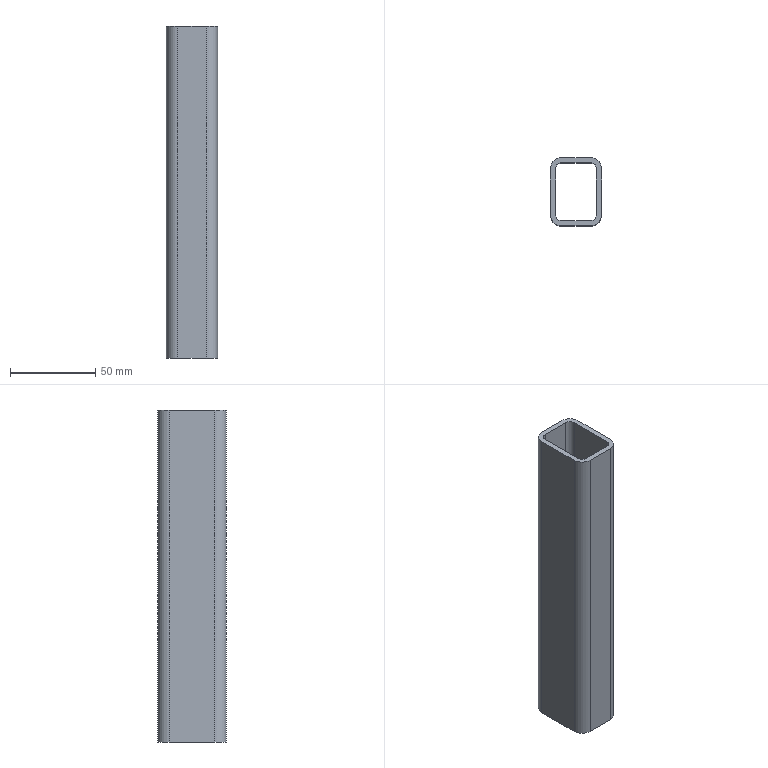Part | STEP file | DIN EN 10305-5 40 x 30 x 3 1785429668101 | 1 solid | 18 faces | box 30 x 40 x 194.434 mm | volume 69555 mm3 | plane 10 | cylinder 8 | commonest cylinder face diameters 7.2 x4 13.2 x4
STEP:
#1=CARTESIAN_POINT('',(-8.4,-17.,194.434));
#2=VERTEX_POINT('',#1);
#3=CARTESIAN_POINT('',(8.4,-17.,194.434));
#4=VERTEX_POINT('',#3);
#5=CARTESIAN_POINT('',(4.2,-17.,194.434));
#6=DIRECTION('',(1.,0.,0.));
#7=VECTOR('',#6,10.);
#8=LINE('',#5,#7);
#9=EDGE_CURVE('',#2,#4,#8,.T.);
#10=ORIENTED_EDGE('',*,*,#9,.T.);
#11=CARTESIAN_POINT('',(8.4,-17.,0.));
#12=VERTEX_POINT('',#11);
#13=CARTESIAN_POINT('',(8.4,-17.,0.));
#14=DIRECTION('',(0.,0.,1.));
#15=VECTOR('',#14,10.);
#16=LINE('',#13,#15);
#17=EDGE_CURVE('',#12,#4,#16,.T.);
#18=ORIENTED_EDGE('',*,*,#17,.F.);
#19=CARTESIAN_POINT('',(-8.4,-17.,0.));
#20=VERTEX_POINT('',#19);
#21=CARTESIAN_POINT('',(4.2,-17.,0.));
#22=DIRECTION('',(1.,0.,0.));
#23=VECTOR('',#22,10.);
#24=LINE('',#21,#23);
#25=EDGE_CURVE('',#20,#12,#24,.T.);
#26=ORIENTED_EDGE('',*,*,#25,.F.);
#27=CARTESIAN_POINT('',(-8.4,-17.,0.));
#28=DIRECTION('',(0.,0.,1.));
#29=VECTOR('',#28,10.);
#30=LINE('',#27,#29);
#31=EDGE_CURVE('',#20,#2,#30,.T.);
#32=ORIENTED_EDGE('',*,*,#31,.T.);
#33=EDGE_LOOP('',(#10,#18,#26,#32));
#34=FACE_OUTER_BOUND('',#33,.T.);
#35=CARTESIAN_POINT('',(8.4,-17.,0.));
#36=DIRECTION('',(0.,-1.,0.));
#37=DIRECTION('',(0.,0.,-1.));
#38=AXIS2_PLACEMENT_3D('',#35,#36,#37);
#39=PLANE('',#38);
#40=ADVANCED_FACE('',(#34),#39,.F.);
#41=CARTESIAN_POINT('',(12.,-13.4,194.434));
#42=VERTEX_POINT('',#41);
#43=CARTESIAN_POINT('',(8.4,-13.4,194.434));
#44=DIRECTION('',(0.,0.,1.));
#45=DIRECTION('',(0.,1.,0.));
#46=AXIS2_PLACEMENT_3D('',#43,#44,#45);
#47=CIRCLE('',#46,3.6);
#48=EDGE_CURVE('',#4,#42,#47,.T.);
#49=ORIENTED_EDGE('',*,*,#48,.T.);
#50=CARTESIAN_POINT('',(12.,-13.4,0.));
#51=VERTEX_POINT('',#50);
#52=CARTESIAN_POINT('',(12.,-13.4,0.));
#53=DIRECTION('',(0.,0.,1.));
#54=VECTOR('',#53,10.);
#55=LINE('',#52,#54);
#56=EDGE_CURVE('',#51,#42,#55,.T.);
#57=ORIENTED_EDGE('',*,*,#56,.F.);
#58=CARTESIAN_POINT('',(8.4,-13.4,0.));
#59=DIRECTION('',(0.,0.,1.));
#60=DIRECTION('',(0.,1.,0.));
#61=AXIS2_PLACEMENT_3D('',#58,#59,#60);
#62=CIRCLE('',#61,3.6);
#63=EDGE_CURVE('',#12,#51,#62,.T.);
#64=ORIENTED_EDGE('',*,*,#63,.F.);
#65=ORIENTED_EDGE('',*,*,#17,.T.);
#66=EDGE_LOOP('',(#49,#57,#64,#65));
#67=FACE_OUTER_BOUND('',#66,.T.);
#68=CARTESIAN_POINT('',(8.4,-13.4,0.));
#69=DIRECTION('',(0.,0.,1.));
#70=DIRECTION('',(0.,1.,0.));
#71=AXIS2_PLACEMENT_3D('',#68,#69,#70);
#72=CYLINDRICAL_SURFACE('',#71,3.6);
#73=ADVANCED_FACE('',(#67),#72,.F.);
#74=CARTESIAN_POINT('',(12.,13.4,194.434));
#75=VERTEX_POINT('',#74);
#76=CARTESIAN_POINT('',(12.,6.7,194.434));
#77=DIRECTION('',(0.,1.,0.));
#78=VECTOR('',#77,10.);
#79=LINE('',#76,#78);
#80=EDGE_CURVE('',#42,#75,#79,.T.);
#81=ORIENTED_EDGE('',*,*,#80,.T.);
#82=CARTESIAN_POINT('',(12.,13.4,0.));
#83=VERTEX_POINT('',#82);
#84=CARTESIAN_POINT('',(12.,13.4,0.));
#85=DIRECTION('',(0.,0.,1.));
#86=VECTOR('',#85,10.);
#87=LINE('',#84,#86);
#88=EDGE_CURVE('',#83,#75,#87,.T.);
#89=ORIENTED_EDGE('',*,*,#88,.F.);
#90=CARTESIAN_POINT('',(12.,6.7,0.));
#91=DIRECTION('',(0.,1.,0.));
#92=VECTOR('',#91,10.);
#93=LINE('',#90,#92);
#94=EDGE_CURVE('',#51,#83,#93,.T.);
#95=ORIENTED_EDGE('',*,*,#94,.F.);
#96=ORIENTED_EDGE('',*,*,#56,.T.);
#97=EDGE_LOOP('',(#81,#89,#95,#96));
#98=FACE_OUTER_BOUND('',#97,.T.);
#99=CARTESIAN_POINT('',(12.,13.4,0.));
#100=DIRECTION('',(1.,0.,0.));
#101=DIRECTION('',(0.,0.,-1.));
#102=AXIS2_PLACEMENT_3D('',#99,#100,#101);
#103=PLANE('',#102);
#104=ADVANCED_FACE('',(#98),#103,.F.);
#105=CARTESIAN_POINT('',(8.4,17.,194.434));
#106=VERTEX_POINT('',#105);
#107=CARTESIAN_POINT('',(8.4,13.4,194.434));
#108=DIRECTION('',(0.,0.,1.));
#109=DIRECTION('',(-1.,0.,0.));
#110=AXIS2_PLACEMENT_3D('',#107,#108,#109);
#111=CIRCLE('',#110,3.6);
#112=EDGE_CURVE('',#75,#106,#111,.T.);
#113=ORIENTED_EDGE('',*,*,#112,.T.);
#114=CARTESIAN_POINT('',(8.4,17.,0.));
#115=VERTEX_POINT('',#114);
#116=CARTESIAN_POINT('',(8.4,17.,0.));
#117=DIRECTION('',(0.,0.,1.));
#118=VECTOR('',#117,10.);
#119=LINE('',#116,#118);
#120=EDGE_CURVE('',#115,#106,#119,.T.);
#121=ORIENTED_EDGE('',*,*,#120,.F.);
#122=CARTESIAN_POINT('',(8.4,13.4,0.));
#123=DIRECTION('',(0.,0.,1.));
#124=DIRECTION('',(-1.,0.,0.));
#125=AXIS2_PLACEMENT_3D('',#122,#123,#124);
#126=CIRCLE('',#125,3.6);
#127=EDGE_CURVE('',#83,#115,#126,.T.);
#128=ORIENTED_EDGE('',*,*,#127,.F.);
#129=ORIENTED_EDGE('',*,*,#88,.T.);
#130=EDGE_LOOP('',(#113,#121,#128,#129));
#131=FACE_OUTER_BOUND('',#130,.T.);
#132=CARTESIAN_POINT('',(8.4,13.4,0.));
#133=DIRECTION('',(0.,0.,1.));
#134=DIRECTION('',(-1.,0.,0.));
#135=AXIS2_PLACEMENT_3D('',#132,#133,#134);
#136=CYLINDRICAL_SURFACE('',#135,3.6);
#137=ADVANCED_FACE('',(#131),#136,.F.);
#138=CARTESIAN_POINT('',(15.,13.4,194.434));
#139=VERTEX_POINT('',#138);
#140=CARTESIAN_POINT('',(15.,-13.4,194.434));
#141=VERTEX_POINT('',#140);
#142=CARTESIAN_POINT('',(15.,6.7,194.434));
#143=DIRECTION('',(0.,-1.,0.));
#144=VECTOR('',#143,10.);
#145=LINE('',#142,#144);
#146=EDGE_CURVE('',#139,#141,#145,.T.);
#147=ORIENTED_EDGE('',*,*,#146,.T.);
#148=CARTESIAN_POINT('',(15.,-13.4,0.));
#149=VERTEX_POINT('',#148);
#150=CARTESIAN_POINT('',(15.,-13.4,0.));
#151=DIRECTION('',(0.,0.,1.));
#152=VECTOR('',#151,10.);
#153=LINE('',#150,#152);
#154=EDGE_CURVE('',#149,#141,#153,.T.);
#155=ORIENTED_EDGE('',*,*,#154,.F.);
#156=CARTESIAN_POINT('',(15.,13.4,0.));
#157=VERTEX_POINT('',#156);
#158=CARTESIAN_POINT('',(15.,6.7,0.));
#159=DIRECTION('',(0.,-1.,0.));
#160=VECTOR('',#159,10.);
#161=LINE('',#158,#160);
#162=EDGE_CURVE('',#157,#149,#161,.T.);
#163=ORIENTED_EDGE('',*,*,#162,.F.);
#164=CARTESIAN_POINT('',(15.,13.4,0.));
#165=DIRECTION('',(0.,0.,1.));
#166=VECTOR('',#165,10.);
#167=LINE('',#164,#166);
#168=EDGE_CURVE('',#157,#139,#167,.T.);
#169=ORIENTED_EDGE('',*,*,#168,.T.);
#170=EDGE_LOOP('',(#147,#155,#163,#169));
#171=FACE_OUTER_BOUND('',#170,.T.);
#172=CARTESIAN_POINT('',(15.,13.4,0.));
#173=DIRECTION('',(1.,0.,0.));
#174=DIRECTION('',(0.,0.,-1.));
#175=AXIS2_PLACEMENT_3D('',#172,#173,#174);
#176=PLANE('',#175);
#177=ADVANCED_FACE('',(#171),#176,.T.);
#178=CARTESIAN_POINT('',(8.4,-20.,194.434));
#179=VERTEX_POINT('',#178);
#180=CARTESIAN_POINT('',(8.4,-13.4,194.434));
#181=DIRECTION('',(0.,0.,-1.));
#182=DIRECTION('',(0.,1.,0.));
#183=AXIS2_PLACEMENT_3D('',#180,#181,#182);
#184=CIRCLE('',#183,6.6);
#185=EDGE_CURVE('',#141,#179,#184,.T.);
#186=ORIENTED_EDGE('',*,*,#185,.T.);
#187=CARTESIAN_POINT('',(8.4,-20.,0.));
#188=VERTEX_POINT('',#187);
#189=CARTESIAN_POINT('',(8.4,-20.,0.));
#190=DIRECTION('',(0.,0.,1.));
#191=VECTOR('',#190,10.);
#192=LINE('',#189,#191);
#193=EDGE_CURVE('',#188,#179,#192,.T.);
#194=ORIENTED_EDGE('',*,*,#193,.F.);
#195=CARTESIAN_POINT('',(8.4,-13.4,0.));
#196=DIRECTION('',(0.,0.,-1.));
#197=DIRECTION('',(0.,1.,0.));
#198=AXIS2_PLACEMENT_3D('',#195,#196,#197);
#199=CIRCLE('',#198,6.6);
#200=EDGE_CURVE('',#149,#188,#199,.T.);
#201=ORIENTED_EDGE('',*,*,#200,.F.);
#202=ORIENTED_EDGE('',*,*,#154,.T.);
#203=EDGE_LOOP('',(#186,#194,#201,#202));
#204=FACE_OUTER_BOUND('',#203,.T.);
#205=CARTESIAN_POINT('',(8.4,-13.4,0.));
#206=DIRECTION('',(0.,0.,1.));
#207=DIRECTION('',(0.,1.,0.));
#208=AXIS2_PLACEMENT_3D('',#205,#206,#207);
#209=CYLINDRICAL_SURFACE('',#208,6.6);
#210=ADVANCED_FACE('',(#204),#209,.T.);
#211=CARTESIAN_POINT('',(-8.4,-20.,194.434));
#212=VERTEX_POINT('',#211);
#213=CARTESIAN_POINT('',(4.2,-20.,194.434));
#214=DIRECTION('',(-1.,0.,0.));
#215=VECTOR('',#214,10.);
#216=LINE('',#213,#215);
#217=EDGE_CURVE('',#179,#212,#216,.T.);
#218=ORIENTED_EDGE('',*,*,#217,.T.);
#219=CARTESIAN_POINT('',(-8.4,-20.,0.));
#220=VERTEX_POINT('',#219);
#221=CARTESIAN_POINT('',(-8.4,-20.,0.));
#222=DIRECTION('',(0.,0.,1.));
#223=VECTOR('',#222,10.);
#224=LINE('',#221,#223);
#225=EDGE_CURVE('',#220,#212,#224,.T.);
#226=ORIENTED_EDGE('',*,*,#225,.F.);
#227=CARTESIAN_POINT('',(4.2,-20.,0.));
#228=DIRECTION('',(-1.,0.,0.));
#229=VECTOR('',#228,10.);
#230=LINE('',#227,#229);
#231=EDGE_CURVE('',#188,#220,#230,.T.);
#232=ORIENTED_EDGE('',*,*,#231,.F.);
#233=ORIENTED_EDGE('',*,*,#193,.T.);
#234=EDGE_LOOP('',(#218,#226,#232,#233));
#235=FACE_OUTER_BOUND('',#234,.T.);
#236=CARTESIAN_POINT('',(8.4,-20.,0.));
#237=DIRECTION('',(0.,-1.,0.));
#238=DIRECTION('',(0.,0.,-1.));
#239=AXIS2_PLACEMENT_3D('',#236,#237,#238);
#240=PLANE('',#239);
#241=ADVANCED_FACE('',(#235),#240,.T.);
#242=CARTESIAN_POINT('',(-15.,-13.4,194.434));
#243=VERTEX_POINT('',#242);
#244=CARTESIAN_POINT('',(-8.4,-13.4,194.434));
#245=DIRECTION('',(0.,0.,-1.));
#246=DIRECTION('',(1.,0.,0.));
#247=AXIS2_PLACEMENT_3D('',#244,#245,#246);
#248=CIRCLE('',#247,6.6);
#249=EDGE_CURVE('',#212,#243,#248,.T.);
#250=ORIENTED_EDGE('',*,*,#249,.T.);
#251=CARTESIAN_POINT('',(-15.,-13.4,0.));
#252=VERTEX_POINT('',#251);
#253=CARTESIAN_POINT('',(-15.,-13.4,0.));
#254=DIRECTION('',(0.,0.,1.));
#255=VECTOR('',#254,10.);
#256=LINE('',#253,#255);
#257=EDGE_CURVE('',#252,#243,#256,.T.);
#258=ORIENTED_EDGE('',*,*,#257,.F.);
#259=CARTESIAN_POINT('',(-8.4,-13.4,0.));
#260=DIRECTION('',(0.,0.,-1.));
#261=DIRECTION('',(1.,0.,0.));
#262=AXIS2_PLACEMENT_3D('',#259,#260,#261);
#263=CIRCLE('',#262,6.6);
#264=EDGE_CURVE('',#220,#252,#263,.T.);
#265=ORIENTED_EDGE('',*,*,#264,.F.);
#266=ORIENTED_EDGE('',*,*,#225,.T.);
#267=EDGE_LOOP('',(#250,#258,#265,#266));
#268=FACE_OUTER_BOUND('',#267,.T.);
#269=CARTESIAN_POINT('',(-8.4,-13.4,0.));
#270=DIRECTION('',(0.,0.,1.));
#271=DIRECTION('',(1.,0.,0.));
#272=AXIS2_PLACEMENT_3D('',#269,#270,#271);
#273=CYLINDRICAL_SURFACE('',#272,6.6);
#274=ADVANCED_FACE('',(#268),#273,.T.);
#275=CARTESIAN_POINT('',(-8.4,17.,194.434));
#276=VERTEX_POINT('',#275);
#277=CARTESIAN_POINT('',(-4.2,17.,194.434));
#278=DIRECTION('',(-1.,0.,0.));
#279=VECTOR('',#278,10.);
#280=LINE('',#277,#279);
#281=EDGE_CURVE('',#106,#276,#280,.T.);
#282=ORIENTED_EDGE('',*,*,#281,.T.);
#283=CARTESIAN_POINT('',(-8.4,17.,0.));
#284=VERTEX_POINT('',#283);
#285=CARTESIAN_POINT('',(-8.4,17.,0.));
#286=DIRECTION('',(0.,0.,1.));
#287=VECTOR('',#286,10.);
#288=LINE('',#285,#287);
#289=EDGE_CURVE('',#284,#276,#288,.T.);
#290=ORIENTED_EDGE('',*,*,#289,.F.);
#291=CARTESIAN_POINT('',(-4.2,17.,0.));
#292=DIRECTION('',(-1.,0.,0.));
#293=VECTOR('',#292,10.);
#294=LINE('',#291,#293);
#295=EDGE_CURVE('',#115,#284,#294,.T.);
#296=ORIENTED_EDGE('',*,*,#295,.F.);
#297=ORIENTED_EDGE('',*,*,#120,.T.);
#298=EDGE_LOOP('',(#282,#290,#296,#297));
#299=FACE_OUTER_BOUND('',#298,.T.);
#300=CARTESIAN_POINT('',(-8.4,17.,0.));
#301=DIRECTION('',(0.,1.,0.));
#302=DIRECTION('',(0.,0.,1.));
#303=AXIS2_PLACEMENT_3D('',#300,#301,#302);
#304=PLANE('',#303);
#305=ADVANCED_FACE('',(#299),#304,.F.);
#306=CARTESIAN_POINT('',(-12.,-13.4,194.434));
#307=VERTEX_POINT('',#306);
#308=CARTESIAN_POINT('',(-8.4,-13.4,194.434));
#309=DIRECTION('',(0.,0.,1.));
#310=DIRECTION('',(1.,0.,0.));
#311=AXIS2_PLACEMENT_3D('',#308,#309,#310);
#312=CIRCLE('',#311,3.6);
#313=EDGE_CURVE('',#307,#2,#312,.T.);
#314=ORIENTED_EDGE('',*,*,#313,.T.);
#315=ORIENTED_EDGE('',*,*,#31,.F.);
#316=CARTESIAN_POINT('',(-12.,-13.4,0.));
#317=VERTEX_POINT('',#316);
#318=CARTESIAN_POINT('',(-8.4,-13.4,0.));
#319=DIRECTION('',(0.,0.,1.));
#320=DIRECTION('',(1.,0.,0.));
#321=AXIS2_PLACEMENT_3D('',#318,#319,#320);
#322=CIRCLE('',#321,3.6);
#323=EDGE_CURVE('',#317,#20,#322,.T.);
#324=ORIENTED_EDGE('',*,*,#323,.F.);
#325=CARTESIAN_POINT('',(-12.,-13.4,0.));
#326=DIRECTION('',(0.,0.,1.));
#327=VECTOR('',#326,10.);
#328=LINE('',#325,#327);
#329=EDGE_CURVE('',#317,#307,#328,.T.);
#330=ORIENTED_EDGE('',*,*,#329,.T.);
#331=EDGE_LOOP('',(#314,#315,#324,#330));
#332=FACE_OUTER_BOUND('',#331,.T.);
#333=CARTESIAN_POINT('',(-8.4,-13.4,0.));
#334=DIRECTION('',(0.,0.,1.));
#335=DIRECTION('',(1.,0.,0.));
#336=AXIS2_PLACEMENT_3D('',#333,#334,#335);
#337=CYLINDRICAL_SURFACE('',#336,3.6);
#338=ADVANCED_FACE('',(#332),#337,.F.);
#339=CARTESIAN_POINT('',(-12.,13.4,194.434));
#340=VERTEX_POINT('',#339);
#341=CARTESIAN_POINT('',(-12.,-6.7,194.434));
#342=DIRECTION('',(0.,-1.,0.));
#343=VECTOR('',#342,10.);
#344=LINE('',#341,#343);
#345=EDGE_CURVE('',#340,#307,#344,.T.);
#346=ORIENTED_EDGE('',*,*,#345,.T.);
#347=ORIENTED_EDGE('',*,*,#329,.F.);
#348=CARTESIAN_POINT('',(-12.,13.4,0.));
#349=VERTEX_POINT('',#348);
#350=CARTESIAN_POINT('',(-12.,-6.7,0.));
#351=DIRECTION('',(0.,-1.,0.));
#352=VECTOR('',#351,10.);
#353=LINE('',#350,#352);
#354=EDGE_CURVE('',#349,#317,#353,.T.);
#355=ORIENTED_EDGE('',*,*,#354,.F.);
#356=CARTESIAN_POINT('',(-12.,13.4,0.));
#357=DIRECTION('',(0.,0.,1.));
#358=VECTOR('',#357,10.);
#359=LINE('',#356,#358);
#360=EDGE_CURVE('',#349,#340,#359,.T.);
#361=ORIENTED_EDGE('',*,*,#360,.T.);
#362=EDGE_LOOP('',(#346,#347,#355,#361));
#363=FACE_OUTER_BOUND('',#362,.T.);
#364=CARTESIAN_POINT('',(-12.,-13.4,0.));
#365=DIRECTION('',(-1.,0.,0.));
#366=DIRECTION('',(0.,0.,1.));
#367=AXIS2_PLACEMENT_3D('',#364,#365,#366);
#368=PLANE('',#367);
#369=ADVANCED_FACE('',(#363),#368,.F.);
#370=CARTESIAN_POINT('',(-8.4,13.4,194.434));
#371=DIRECTION('',(0.,0.,1.));
#372=DIRECTION('',(0.,-1.,0.));
#373=AXIS2_PLACEMENT_3D('',#370,#371,#372);
#374=CIRCLE('',#373,3.6);
#375=EDGE_CURVE('',#276,#340,#374,.T.);
#376=ORIENTED_EDGE('',*,*,#375,.T.);
#377=ORIENTED_EDGE('',*,*,#360,.F.);
#378=CARTESIAN_POINT('',(-8.4,13.4,0.));
#379=DIRECTION('',(0.,0.,1.));
#380=DIRECTION('',(0.,-1.,0.));
#381=AXIS2_PLACEMENT_3D('',#378,#379,#380);
#382=CIRCLE('',#381,3.6);
#383=EDGE_CURVE('',#284,#349,#382,.T.);
#384=ORIENTED_EDGE('',*,*,#383,.F.);
#385=ORIENTED_EDGE('',*,*,#289,.T.);
#386=EDGE_LOOP('',(#376,#377,#384,#385));
#387=FACE_OUTER_BOUND('',#386,.T.);
#388=CARTESIAN_POINT('',(-8.4,13.4,0.));
#389=DIRECTION('',(0.,0.,1.));
#390=DIRECTION('',(0.,-1.,0.));
#391=AXIS2_PLACEMENT_3D('',#388,#389,#390);
#392=CYLINDRICAL_SURFACE('',#391,3.6);
#393=ADVANCED_FACE('',(#387),#392,.F.);
#394=CARTESIAN_POINT('',(-15.,13.4,194.434));
#395=VERTEX_POINT('',#394);
#396=CARTESIAN_POINT('',(-15.,-6.7,194.434));
#397=DIRECTION('',(0.,1.,0.));
#398=VECTOR('',#397,10.);
#399=LINE('',#396,#398);
#400=EDGE_CURVE('',#243,#395,#399,.T.);
#401=ORIENTED_EDGE('',*,*,#400,.T.);
#402=CARTESIAN_POINT('',(-15.,13.4,0.));
#403=VERTEX_POINT('',#402);
#404=CARTESIAN_POINT('',(-15.,13.4,0.));
#405=DIRECTION('',(0.,0.,1.));
#406=VECTOR('',#405,10.);
#407=LINE('',#404,#406);
#408=EDGE_CURVE('',#403,#395,#407,.T.);
#409=ORIENTED_EDGE('',*,*,#408,.F.);
#410=CARTESIAN_POINT('',(-15.,-6.7,0.));
#411=DIRECTION('',(0.,1.,0.));
#412=VECTOR('',#411,10.);
#413=LINE('',#410,#412);
#414=EDGE_CURVE('',#252,#403,#413,.T.);
#415=ORIENTED_EDGE('',*,*,#414,.F.);
#416=ORIENTED_EDGE('',*,*,#257,.T.);
#417=EDGE_LOOP('',(#401,#409,#415,#416));
#418=FACE_OUTER_BOUND('',#417,.T.);
#419=CARTESIAN_POINT('',(-15.,-13.4,0.));
#420=DIRECTION('',(-1.,0.,0.));
#421=DIRECTION('',(0.,0.,1.));
#422=AXIS2_PLACEMENT_3D('',#419,#420,#421);
#423=PLANE('',#422);
#424=ADVANCED_FACE('',(#418),#423,.T.);
#425=CARTESIAN_POINT('',(-8.4,20.,194.434));
#426=VERTEX_POINT('',#425);
#427=CARTESIAN_POINT('',(-8.4,13.4,194.434));
#428=DIRECTION('',(0.,0.,-1.));
#429=DIRECTION('',(0.,-1.,0.));
#430=AXIS2_PLACEMENT_3D('',#427,#428,#429);
#431=CIRCLE('',#430,6.6);
#432=EDGE_CURVE('',#395,#426,#431,.T.);
#433=ORIENTED_EDGE('',*,*,#432,.T.);
#434=CARTESIAN_POINT('',(-8.4,20.,0.));
#435=VERTEX_POINT('',#434);
#436=CARTESIAN_POINT('',(-8.4,20.,0.));
#437=DIRECTION('',(0.,0.,1.));
#438=VECTOR('',#437,10.);
#439=LINE('',#436,#438);
#440=EDGE_CURVE('',#435,#426,#439,.T.);
#441=ORIENTED_EDGE('',*,*,#440,.F.);
#442=CARTESIAN_POINT('',(-8.4,13.4,0.));
#443=DIRECTION('',(0.,0.,-1.));
#444=DIRECTION('',(0.,-1.,0.));
#445=AXIS2_PLACEMENT_3D('',#442,#443,#444);
#446=CIRCLE('',#445,6.6);
#447=EDGE_CURVE('',#403,#435,#446,.T.);
#448=ORIENTED_EDGE('',*,*,#447,.F.);
#449=ORIENTED_EDGE('',*,*,#408,.T.);
#450=EDGE_LOOP('',(#433,#441,#448,#449));
#451=FACE_OUTER_BOUND('',#450,.T.);
#452=CARTESIAN_POINT('',(-8.4,13.4,0.));
#453=DIRECTION('',(0.,0.,1.));
#454=DIRECTION('',(0.,-1.,0.));
#455=AXIS2_PLACEMENT_3D('',#452,#453,#454);
#456=CYLINDRICAL_SURFACE('',#455,6.6);
#457=ADVANCED_FACE('',(#451),#456,.T.);
#458=CARTESIAN_POINT('',(8.4,20.,194.434));
#459=VERTEX_POINT('',#458);
#460=CARTESIAN_POINT('',(-4.2,20.,194.434));
#461=DIRECTION('',(1.,0.,0.));
#462=VECTOR('',#461,10.);
#463=LINE('',#460,#462);
#464=EDGE_CURVE('',#426,#459,#463,.T.);
#465=ORIENTED_EDGE('',*,*,#464,.T.);
#466=CARTESIAN_POINT('',(8.4,20.,0.));
#467=VERTEX_POINT('',#466);
#468=CARTESIAN_POINT('',(8.4,20.,0.));
#469=DIRECTION('',(0.,0.,1.));
#470=VECTOR('',#469,10.);
#471=LINE('',#468,#470);
#472=EDGE_CURVE('',#467,#459,#471,.T.);
#473=ORIENTED_EDGE('',*,*,#472,.F.);
#474=CARTESIAN_POINT('',(-4.2,20.,0.));
#475=DIRECTION('',(1.,0.,0.));
#476=VECTOR('',#475,10.);
#477=LINE('',#474,#476);
#478=EDGE_CURVE('',#435,#467,#477,.T.);
#479=ORIENTED_EDGE('',*,*,#478,.F.);
#480=ORIENTED_EDGE('',*,*,#440,.T.);
#481=EDGE_LOOP('',(#465,#473,#479,#480));
#482=FACE_OUTER_BOUND('',#481,.T.);
#483=CARTESIAN_POINT('',(-8.4,20.,0.));
#484=DIRECTION('',(0.,1.,0.));
#485=DIRECTION('',(0.,0.,1.));
#486=AXIS2_PLACEMENT_3D('',#483,#484,#485);
#487=PLANE('',#486);
#488=ADVANCED_FACE('',(#482),#487,.T.);
#489=CARTESIAN_POINT('',(8.4,13.4,194.434));
#490=DIRECTION('',(0.,0.,-1.));
#491=DIRECTION('',(-1.,0.,0.));
#492=AXIS2_PLACEMENT_3D('',#489,#490,#491);
#493=CIRCLE('',#492,6.6);
#494=EDGE_CURVE('',#459,#139,#493,.T.);
#495=ORIENTED_EDGE('',*,*,#494,.T.);
#496=ORIENTED_EDGE('',*,*,#168,.F.);
#497=CARTESIAN_POINT('',(8.4,13.4,0.));
#498=DIRECTION('',(0.,0.,-1.));
#499=DIRECTION('',(-1.,0.,0.));
#500=AXIS2_PLACEMENT_3D('',#497,#498,#499);
#501=CIRCLE('',#500,6.6);
#502=EDGE_CURVE('',#467,#157,#501,.T.);
#503=ORIENTED_EDGE('',*,*,#502,.F.);
#504=ORIENTED_EDGE('',*,*,#472,.T.);
#505=EDGE_LOOP('',(#495,#496,#503,#504));
#506=FACE_OUTER_BOUND('',#505,.T.);
#507=CARTESIAN_POINT('',(8.4,13.4,0.));
#508=DIRECTION('',(0.,0.,1.));
#509=DIRECTION('',(-1.,0.,0.));
#510=AXIS2_PLACEMENT_3D('',#507,#508,#509);
#511=CYLINDRICAL_SURFACE('',#510,6.6);
#512=ADVANCED_FACE('',(#506),#511,.T.);
#513=ORIENTED_EDGE('',*,*,#414,.T.);
#514=ORIENTED_EDGE('',*,*,#447,.T.);
#515=ORIENTED_EDGE('',*,*,#478,.T.);
#516=ORIENTED_EDGE('',*,*,#502,.T.);
#517=ORIENTED_EDGE('',*,*,#162,.T.);
#518=ORIENTED_EDGE('',*,*,#200,.T.);
#519=ORIENTED_EDGE('',*,*,#231,.T.);
#520=ORIENTED_EDGE('',*,*,#264,.T.);
#521=EDGE_LOOP('',(#513,#514,#515,#516,#517,#518,#519,#520));
#522=FACE_OUTER_BOUND('',#521,.T.);
#523=ORIENTED_EDGE('',*,*,#295,.T.);
#524=ORIENTED_EDGE('',*,*,#383,.T.);
#525=ORIENTED_EDGE('',*,*,#354,.T.);
#526=ORIENTED_EDGE('',*,*,#323,.T.);
#527=ORIENTED_EDGE('',*,*,#25,.T.);
#528=ORIENTED_EDGE('',*,*,#63,.T.);
#529=ORIENTED_EDGE('',*,*,#94,.T.);
#530=ORIENTED_EDGE('',*,*,#127,.T.);
#531=EDGE_LOOP('',(#523,#524,#525,#526,#527,#528,#529,#530));
#532=FACE_BOUND('',#531,.T.);
#533=CARTESIAN_POINT('',(0.,0.,0.));
#534=DIRECTION('',(0.,0.,1.));
#535=DIRECTION('',(1.,0.,0.));
#536=AXIS2_PLACEMENT_3D('',#533,#534,#535);
#537=PLANE('',#536);
#538=ADVANCED_FACE('',(#522,#532),#537,.F.);
#539=ORIENTED_EDGE('',*,*,#400,.F.);
#540=ORIENTED_EDGE('',*,*,#249,.F.);
#541=ORIENTED_EDGE('',*,*,#217,.F.);
#542=ORIENTED_EDGE('',*,*,#185,.F.);
#543=ORIENTED_EDGE('',*,*,#146,.F.);
#544=ORIENTED_EDGE('',*,*,#494,.F.);
#545=ORIENTED_EDGE('',*,*,#464,.F.);
#546=ORIENTED_EDGE('',*,*,#432,.F.);
#547=EDGE_LOOP('',(#539,#540,#541,#542,#543,#544,#545,#546));
#548=FACE_OUTER_BOUND('',#547,.T.);
#549=ORIENTED_EDGE('',*,*,#281,.F.);
#550=ORIENTED_EDGE('',*,*,#112,.F.);
#551=ORIENTED_EDGE('',*,*,#80,.F.);
#552=ORIENTED_EDGE('',*,*,#48,.F.);
#553=ORIENTED_EDGE('',*,*,#9,.F.);
#554=ORIENTED_EDGE('',*,*,#313,.F.);
#555=ORIENTED_EDGE('',*,*,#345,.F.);
#556=ORIENTED_EDGE('',*,*,#375,.F.);
#557=EDGE_LOOP('',(#549,#550,#551,#552,#553,#554,#555,#556));
#558=FACE_BOUND('',#557,.T.);
#559=CARTESIAN_POINT('',(0.,0.,194.434));
#560=DIRECTION('',(0.,0.,1.));
#561=DIRECTION('',(1.,0.,0.));
#562=AXIS2_PLACEMENT_3D('',#559,#560,#561);
#563=PLANE('',#562);
#564=ADVANCED_FACE('',(#548,#558),#563,.T.);
#565=CLOSED_SHELL('',(#40,#73,#104,#137,#177,#210,#241,#274,#305,#338,#369,#393,#424,#457,#488,#512,#538,#564));
#566=MANIFOLD_SOLID_BREP('',#565);
#567=(LENGTH_UNIT()NAMED_UNIT(*)SI_UNIT(.MILLI.,.METRE.));
#568=UNCERTAINTY_MEASURE_WITH_UNIT(LENGTH_MEASURE(0.01),#567,'','');
#569=(NAMED_UNIT(*)PLANE_ANGLE_UNIT()SI_UNIT($,.RADIAN.));
#570=(NAMED_UNIT(*)SI_UNIT($,.STERADIAN.)SOLID_ANGLE_UNIT());
#571=(GEOMETRIC_REPRESENTATION_CONTEXT(3)GLOBAL_UNCERTAINTY_ASSIGNED_CONTEXT((#568))GLOBAL_UNIT_ASSIGNED_CONTEXT((#567,#569,#570))REPRESENTATION_CONTEXT('',''));
#572=ADVANCED_BREP_SHAPE_REPRESENTATION('',(#566),#571);